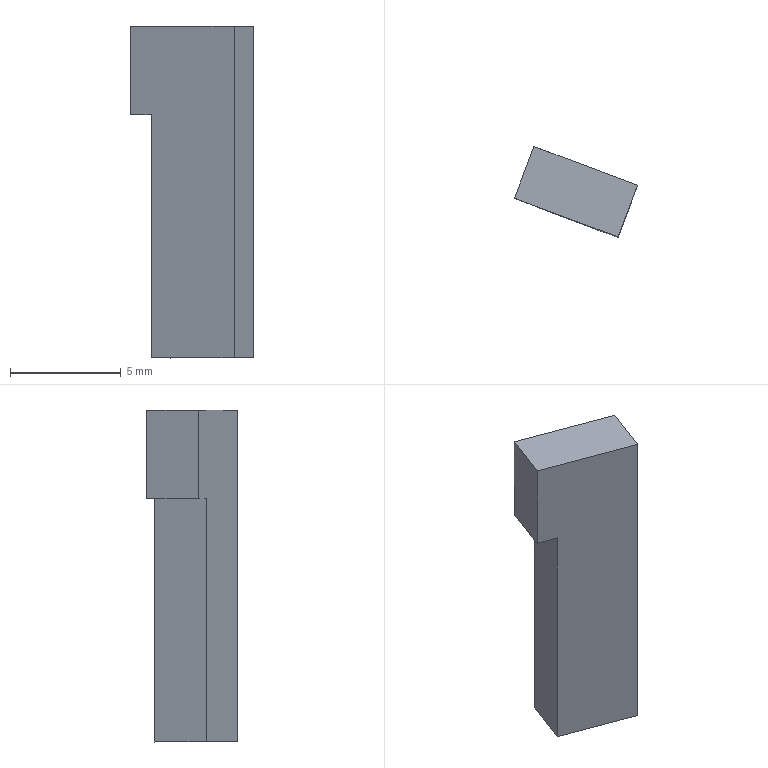Part | NX | features 13 2 | 1 solid | 8 faces | box 5.559 x 4.093 x 15 mm | volume 160 mm3 | plane 8
STEP:
#1=CARTESIAN_POINT('',(358.001,46.466,0.002111));
#2=VERTEX_POINT('',#1);
#3=CARTESIAN_POINT('',(357.125,44.124,0.002111));
#4=VERTEX_POINT('',#3);
#5=CARTESIAN_POINT('',(360.101,52.082,0.002111));
#6=DIRECTION('',(-0.3502,-0.9367,0.000000001));
#7=VECTOR('',#6,1000.);
#8=LINE('',#5,#7);
#9=EDGE_CURVE('',#2,#4,#8,.T.);
#10=ORIENTED_EDGE('',*,*,#9,.T.);
#11=CARTESIAN_POINT('',(353.378,45.525,0.002031));
#12=VERTEX_POINT('',#11);
#13=CARTESIAN_POINT('',(355.252,44.825,0.002071));
#14=DIRECTION('',(-0.9367,0.3502,-0.00001998));
#15=VECTOR('',#14,1000.);
#16=LINE('',#13,#15);
#17=EDGE_CURVE('',#4,#12,#16,.T.);
#18=ORIENTED_EDGE('',*,*,#17,.T.);
#19=CARTESIAN_POINT('',(354.254,47.867,0.002031));
#20=VERTEX_POINT('',#19);
#21=CARTESIAN_POINT('',(356.354,53.483,0.002031));
#22=DIRECTION('',(0.3502,0.9367,-0.000000001));
#23=VECTOR('',#22,1000.);
#24=LINE('',#21,#23);
#25=EDGE_CURVE('',#12,#20,#24,.T.);
#26=ORIENTED_EDGE('',*,*,#25,.T.);
#27=CARTESIAN_POINT('',(356.127,47.166,0.002071));
#28=DIRECTION('',(0.9367,-0.3502,0.00001998));
#29=VECTOR('',#28,1000.);
#30=LINE('',#27,#29);
#31=EDGE_CURVE('',#20,#2,#30,.T.);
#32=ORIENTED_EDGE('',*,*,#31,.T.);
#33=EDGE_LOOP('',(#10,#18,#26,#32));
#34=FACE_BOUND('',#33,.T.);
#35=CARTESIAN_POINT('',(358.227,52.783,0.002071));
#36=DIRECTION('',(-0.00001871,0.000006998,1.));
#37=DIRECTION('',(0.9172,-0.3985,0.00001995));
#38=AXIS2_PLACEMENT_3D('',#35,#36,#37);
#39=PLANE('',#38);
#40=ADVANCED_FACE('',(#34),#39,.F.);
#41=CARTESIAN_POINT('',(354.254,47.867,11.002));
#42=VERTEX_POINT('',#41);
#43=CARTESIAN_POINT('',(353.317,48.217,11.002));
#44=VERTEX_POINT('',#43);
#45=CARTESIAN_POINT('',(356.127,47.167,11.002));
#46=DIRECTION('',(-0.9367,0.3502,-0.00001998));
#47=VECTOR('',#46,1000.);
#48=LINE('',#45,#47);
#49=EDGE_CURVE('',#42,#44,#48,.T.);
#50=ORIENTED_EDGE('',*,*,#49,.F.);
#51=CARTESIAN_POINT('',(353.378,45.525,11.002));
#52=VERTEX_POINT('',#51);
#53=CARTESIAN_POINT('',(354.254,47.867,11.002));
#54=DIRECTION('',(-0.3502,-0.9367,0.000000001));
#55=VECTOR('',#54,1000.);
#56=LINE('',#53,#55);
#57=EDGE_CURVE('',#42,#52,#56,.T.);
#58=ORIENTED_EDGE('',*,*,#57,.T.);
#59=CARTESIAN_POINT('',(352.442,45.875,11.002));
#60=VERTEX_POINT('',#59);
#61=CARTESIAN_POINT('',(355.252,44.825,11.002));
#62=DIRECTION('',(0.9367,-0.3502,0.00001998));
#63=VECTOR('',#62,1000.);
#64=LINE('',#61,#63);
#65=EDGE_CURVE('',#60,#52,#64,.T.);
#66=ORIENTED_EDGE('',*,*,#65,.F.);
#67=CARTESIAN_POINT('',(353.317,48.217,11.002));
#68=DIRECTION('',(0.3502,0.9367,-0.000000001));
#69=VECTOR('',#68,1000.);
#70=LINE('',#67,#69);
#71=EDGE_CURVE('',#60,#44,#70,.T.);
#72=ORIENTED_EDGE('',*,*,#71,.T.);
#73=EDGE_LOOP('',(#50,#58,#66,#72));
#74=FACE_BOUND('',#73,.T.);
#75=CARTESIAN_POINT('',(357.351,50.441,11.002));
#76=DIRECTION('',(0.00001871,-0.000006998,-1.));
#77=DIRECTION('',(0.9367,-0.3502,0.00001998));
#78=AXIS2_PLACEMENT_3D('',#75,#76,#77);
#79=PLANE('',#78);
#80=ADVANCED_FACE('',(#74),#79,.T.);
#81=CARTESIAN_POINT('',(357.125,44.124,15.002));
#82=VERTEX_POINT('',#81);
#83=CARTESIAN_POINT('',(358.,46.466,15.002));
#84=VERTEX_POINT('',#83);
#85=CARTESIAN_POINT('',(358.,46.466,15.002));
#86=DIRECTION('',(0.3502,0.9367,-0.000000001));
#87=VECTOR('',#86,1000.);
#88=LINE('',#85,#87);
#89=EDGE_CURVE('',#82,#84,#88,.T.);
#90=ORIENTED_EDGE('',*,*,#89,.T.);
#91=CARTESIAN_POINT('',(353.317,48.217,15.002));
#92=VERTEX_POINT('',#91);
#93=CARTESIAN_POINT('',(356.127,47.167,15.002));
#94=DIRECTION('',(0.9367,-0.3502,0.00001998));
#95=VECTOR('',#94,1000.);
#96=LINE('',#93,#95);
#97=EDGE_CURVE('',#92,#84,#96,.T.);
#98=ORIENTED_EDGE('',*,*,#97,.F.);
#99=CARTESIAN_POINT('',(352.442,45.875,15.002));
#100=VERTEX_POINT('',#99);
#101=CARTESIAN_POINT('',(353.317,48.217,15.002));
#102=DIRECTION('',(0.3502,0.9367,-0.000000001));
#103=VECTOR('',#102,1000.);
#104=LINE('',#101,#103);
#105=EDGE_CURVE('',#100,#92,#104,.T.);
#106=ORIENTED_EDGE('',*,*,#105,.F.);
#107=CARTESIAN_POINT('',(355.252,44.825,15.002));
#108=DIRECTION('',(-0.9367,0.3502,-0.00001998));
#109=VECTOR('',#108,1000.);
#110=LINE('',#107,#109);
#111=EDGE_CURVE('',#82,#100,#110,.T.);
#112=ORIENTED_EDGE('',*,*,#111,.F.);
#113=EDGE_LOOP('',(#90,#98,#106,#112));
#114=FACE_BOUND('',#113,.T.);
#115=CARTESIAN_POINT('',(358.227,52.783,15.002));
#116=DIRECTION('',(0.00001871,-0.000006998,-1.));
#117=DIRECTION('',(-0.9172,0.3985,-0.00001995));
#118=AXIS2_PLACEMENT_3D('',#115,#116,#117);
#119=PLANE('',#118);
#120=ADVANCED_FACE('',(#114),#119,.F.);
#121=CARTESIAN_POINT('',(357.125,44.124,-0.3522));
#122=DIRECTION('',(-0.00001871,0.000006998,1.));
#123=VECTOR('',#122,1000.);
#124=LINE('',#121,#123);
#125=EDGE_CURVE('',#4,#82,#124,.T.);
#126=ORIENTED_EDGE('',*,*,#125,.F.);
#127=ORIENTED_EDGE('',*,*,#9,.F.);
#128=CARTESIAN_POINT('',(358.001,46.466,-0.3503));
#129=DIRECTION('',(-0.00001871,0.000006998,1.));
#130=VECTOR('',#129,1000.);
#131=LINE('',#128,#130);
#132=EDGE_CURVE('',#2,#84,#131,.T.);
#133=ORIENTED_EDGE('',*,*,#132,.T.);
#134=ORIENTED_EDGE('',*,*,#89,.F.);
#135=EDGE_LOOP('',(#126,#127,#133,#134));
#136=FACE_BOUND('',#135,.T.);
#137=CARTESIAN_POINT('',(358.001,46.466,-0.3503));
#138=DIRECTION('',(-0.9367,0.3502,-0.00001998));
#139=DIRECTION('',(-0.3502,-0.9367,0.000000001));
#140=AXIS2_PLACEMENT_3D('',#137,#138,#139);
#141=PLANE('',#140);
#142=ADVANCED_FACE('',(#136),#141,.F.);
#143=ORIENTED_EDGE('',*,*,#132,.F.);
#144=ORIENTED_EDGE('',*,*,#31,.F.);
#145=CARTESIAN_POINT('',(354.254,47.867,-0.3505));
#146=DIRECTION('',(-0.00001871,0.000006998,1.));
#147=VECTOR('',#146,1000.);
#148=LINE('',#145,#147);
#149=EDGE_CURVE('',#20,#42,#148,.T.);
#150=ORIENTED_EDGE('',*,*,#149,.T.);
#151=ORIENTED_EDGE('',*,*,#49,.T.);
#152=CARTESIAN_POINT('',(353.317,48.217,-0.3504));
#153=DIRECTION('',(-0.00001871,0.000006998,1.));
#154=VECTOR('',#153,1000.);
#155=LINE('',#152,#154);
#156=EDGE_CURVE('',#44,#92,#155,.T.);
#157=ORIENTED_EDGE('',*,*,#156,.T.);
#158=ORIENTED_EDGE('',*,*,#97,.T.);
#159=EDGE_LOOP('',(#143,#144,#150,#151,#157,#158));
#160=FACE_BOUND('',#159,.T.);
#161=CARTESIAN_POINT('',(356.127,47.166,-0.3504));
#162=DIRECTION('',(-0.3502,-0.9367,0.000000001));
#163=DIRECTION('',(0.9367,-0.3502,0.00001998));
#164=AXIS2_PLACEMENT_3D('',#161,#162,#163);
#165=PLANE('',#164);
#166=ADVANCED_FACE('',(#160),#165,.F.);
#167=ORIENTED_EDGE('',*,*,#71,.F.);
#168=CARTESIAN_POINT('',(352.442,45.875,-0.3505));
#169=DIRECTION('',(-0.00001871,0.000006998,1.));
#170=VECTOR('',#169,1000.);
#171=LINE('',#168,#170);
#172=EDGE_CURVE('',#60,#100,#171,.T.);
#173=ORIENTED_EDGE('',*,*,#172,.T.);
#174=ORIENTED_EDGE('',*,*,#105,.T.);
#175=ORIENTED_EDGE('',*,*,#156,.F.);
#176=EDGE_LOOP('',(#167,#173,#174,#175));
#177=FACE_BOUND('',#176,.T.);
#178=CARTESIAN_POINT('',(353.317,48.217,-0.3505));
#179=DIRECTION('',(0.9367,-0.3502,0.00001998));
#180=DIRECTION('',(0.3502,0.9367,-0.000000001));
#181=AXIS2_PLACEMENT_3D('',#178,#179,#180);
#182=PLANE('',#181);
#183=ADVANCED_FACE('',(#177),#182,.F.);
#184=ORIENTED_EDGE('',*,*,#65,.T.);
#185=CARTESIAN_POINT('',(353.378,45.525,-0.3524));
#186=DIRECTION('',(-0.00001871,0.000006998,1.));
#187=VECTOR('',#186,1000.);
#188=LINE('',#185,#187);
#189=EDGE_CURVE('',#12,#52,#188,.T.);
#190=ORIENTED_EDGE('',*,*,#189,.F.);
#191=ORIENTED_EDGE('',*,*,#17,.F.);
#192=ORIENTED_EDGE('',*,*,#125,.T.);
#193=ORIENTED_EDGE('',*,*,#111,.T.);
#194=ORIENTED_EDGE('',*,*,#172,.F.);
#195=EDGE_LOOP('',(#184,#190,#191,#192,#193,#194));
#196=FACE_BOUND('',#195,.T.);
#197=CARTESIAN_POINT('',(355.252,44.825,-0.3523));
#198=DIRECTION('',(0.3502,0.9367,-0.000000001));
#199=DIRECTION('',(-0.9367,0.3502,-0.00001998));
#200=AXIS2_PLACEMENT_3D('',#197,#198,#199);
#201=PLANE('',#200);
#202=ADVANCED_FACE('',(#196),#201,.F.);
#203=ORIENTED_EDGE('',*,*,#189,.T.);
#204=ORIENTED_EDGE('',*,*,#57,.F.);
#205=ORIENTED_EDGE('',*,*,#149,.F.);
#206=ORIENTED_EDGE('',*,*,#25,.F.);
#207=EDGE_LOOP('',(#203,#204,#205,#206));
#208=FACE_BOUND('',#207,.T.);
#209=CARTESIAN_POINT('',(354.254,47.867,-0.3505));
#210=DIRECTION('',(0.9367,-0.3502,0.00001998));
#211=DIRECTION('',(0.3502,0.9367,-0.000000001));
#212=AXIS2_PLACEMENT_3D('',#209,#210,#211);
#213=PLANE('',#212);
#214=ADVANCED_FACE('',(#208),#213,.F.);
#215=CLOSED_SHELL('',(#40,#80,#120,#142,#166,#183,#202,#214));
#216=MANIFOLD_SOLID_BREP('',#215);
#217=(LENGTH_UNIT()NAMED_UNIT(*)SI_UNIT(.MILLI.,.METRE.));
#218=UNCERTAINTY_MEASURE_WITH_UNIT(LENGTH_MEASURE(0.00001),#217,'','');
#219=(NAMED_UNIT(*)PLANE_ANGLE_UNIT()SI_UNIT($,.RADIAN.));
#220=(NAMED_UNIT(*)SI_UNIT($,.STERADIAN.)SOLID_ANGLE_UNIT());
#221=(GEOMETRIC_REPRESENTATION_CONTEXT(3)GLOBAL_UNCERTAINTY_ASSIGNED_CONTEXT((#218))GLOBAL_UNIT_ASSIGNED_CONTEXT((#217,#219,#220))REPRESENTATION_CONTEXT('',''));
#222=ADVANCED_BREP_SHAPE_REPRESENTATION('',(#216),#221);